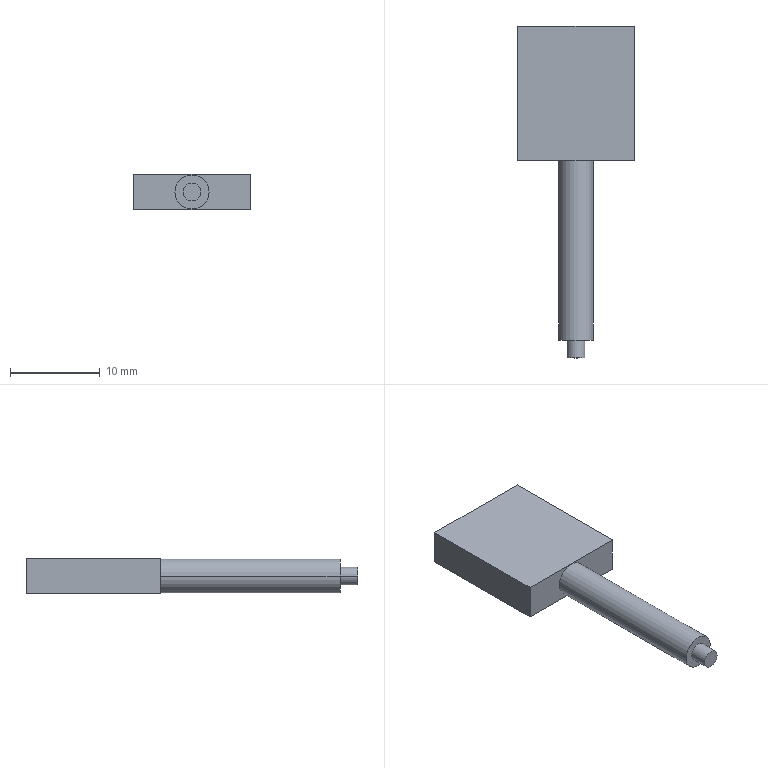Part | STEP file | 0246_008_FPCN14H-1 | 1 solid | 17 faces | box 13 x 37 x 4 mm | volume 994.356 mm3 | plane 13 | cylinder 4 | commonest cylinder face diameters 2 x2 3.8 x2
STEP:
#1=CARTESIAN_POINT('',(0.,0.,0.));
#2=DIRECTION('',(0.,0.,1.));
#3=DIRECTION('',(1.,0.,0.));
#4=AXIS2_PLACEMENT_3D('',#1,#2,#3);
#5=CARTESIAN_POINT('',(1.,-37.,0.));
#6=VERTEX_POINT('',#5);
#7=CARTESIAN_POINT('',(-1.,-37.,0.));
#8=VERTEX_POINT('',#7);
#9=CARTESIAN_POINT('',(0.,-37.,0.));
#10=DIRECTION('',(0.,-1.,0.));
#11=DIRECTION('',(1.,0.,0.));
#12=AXIS2_PLACEMENT_3D('',#9,#10,#11);
#13=CIRCLE('',#12,1.);
#14=CARTESIAN_POINT('',(0.,-37.,0.));
#15=DIRECTION('',(0.,1.,0.));
#16=DIRECTION('',(-1.,0.,0.));
#17=AXIS2_PLACEMENT_3D('',#14,#15,#16);
#18=CYLINDRICAL_SURFACE('',#17,1.);
#19=CARTESIAN_POINT('',(3.142,0.));
#20=DIRECTION('',(-1.,0.));
#21=VECTOR('',#20,1.);
#22=LINE('',#19,#21);
#23=(GEOMETRIC_REPRESENTATION_CONTEXT(2)PARAMETRIC_REPRESENTATION_CONTEXT()REPRESENTATION_CONTEXT('',''));
#24=DEFINITIONAL_REPRESENTATION('',(#22),#23);
#25=PCURVE('',#18,#24);
#26=CARTESIAN_POINT('',(0.,-37.,0.));
#27=DIRECTION('',(0.,-1.,0.));
#28=DIRECTION('',(1.,0.,0.));
#29=AXIS2_PLACEMENT_3D('',#26,#27,#28);
#30=PLANE('',#29);
#31=CARTESIAN_POINT('',(0.,0.));
#32=DIRECTION('',(1.,0.));
#33=AXIS2_PLACEMENT_2D('',#31,#32);
#34=CIRCLE('',#33,1.);
#35=(GEOMETRIC_REPRESENTATION_CONTEXT(2)PARAMETRIC_REPRESENTATION_CONTEXT()REPRESENTATION_CONTEXT('',''));
#36=DEFINITIONAL_REPRESENTATION('',(#34),#35);
#37=PCURVE('',#30,#36);
#38=SURFACE_CURVE('',#13,(#25,#37),.PCURVE_S1.);
#39=EDGE_CURVE('',#6,#8,#38,.T.);
#40=ORIENTED_EDGE('',*,*,#39,.F.);
#41=CARTESIAN_POINT('',(1.,-35.,0.));
#42=VERTEX_POINT('',#41);
#43=CARTESIAN_POINT('',(1.,-37.,0.));
#44=DIRECTION('',(0.,1.,0.));
#45=VECTOR('',#44,1.);
#46=LINE('',#43,#45);
#47=CARTESIAN_POINT('',(3.142,0.));
#48=DIRECTION('',(0.,1.));
#49=VECTOR('',#48,1.);
#50=LINE('',#47,#49);
#51=(GEOMETRIC_REPRESENTATION_CONTEXT(2)PARAMETRIC_REPRESENTATION_CONTEXT()REPRESENTATION_CONTEXT('',''));
#52=DEFINITIONAL_REPRESENTATION('',(#50),#51);
#53=PCURVE('',#18,#52);
#54=CARTESIAN_POINT('',(0.,-37.,0.));
#55=DIRECTION('',(0.,1.,0.));
#56=DIRECTION('',(-1.,0.,0.));
#57=AXIS2_PLACEMENT_3D('',#54,#55,#56);
#58=CYLINDRICAL_SURFACE('',#57,1.);
#59=CARTESIAN_POINT('',(3.142,0.));
#60=DIRECTION('',(0.,1.));
#61=VECTOR('',#60,1.);
#62=LINE('',#59,#61);
#63=(GEOMETRIC_REPRESENTATION_CONTEXT(2)PARAMETRIC_REPRESENTATION_CONTEXT()REPRESENTATION_CONTEXT('',''));
#64=DEFINITIONAL_REPRESENTATION('',(#62),#63);
#65=PCURVE('',#58,#64);
#66=SURFACE_CURVE('',#46,(#53,#65),.PCURVE_S1.);
#67=EDGE_CURVE('',#6,#42,#66,.T.);
#68=ORIENTED_EDGE('',*,*,#67,.T.);
#69=CARTESIAN_POINT('',(-1.,-35.,0.));
#70=VERTEX_POINT('',#69);
#71=CARTESIAN_POINT('',(0.,-35.,0.));
#72=DIRECTION('',(0.,-1.,0.));
#73=DIRECTION('',(1.,0.,0.));
#74=AXIS2_PLACEMENT_3D('',#71,#72,#73);
#75=CIRCLE('',#74,1.);
#76=CARTESIAN_POINT('',(3.142,2.));
#77=DIRECTION('',(-1.,0.));
#78=VECTOR('',#77,1.);
#79=LINE('',#76,#78);
#80=(GEOMETRIC_REPRESENTATION_CONTEXT(2)PARAMETRIC_REPRESENTATION_CONTEXT()REPRESENTATION_CONTEXT('',''));
#81=DEFINITIONAL_REPRESENTATION('',(#79),#80);
#82=PCURVE('',#18,#81);
#83=CARTESIAN_POINT('',(0.,-35.,0.));
#84=DIRECTION('',(0.,-1.,0.));
#85=DIRECTION('',(1.,0.,0.));
#86=AXIS2_PLACEMENT_3D('',#83,#84,#85);
#87=PLANE('',#86);
#88=CARTESIAN_POINT('',(0.,0.));
#89=DIRECTION('',(1.,0.));
#90=AXIS2_PLACEMENT_2D('',#88,#89);
#91=CIRCLE('',#90,1.);
#92=(GEOMETRIC_REPRESENTATION_CONTEXT(2)PARAMETRIC_REPRESENTATION_CONTEXT()REPRESENTATION_CONTEXT('',''));
#93=DEFINITIONAL_REPRESENTATION('',(#91),#92);
#94=PCURVE('',#87,#93);
#95=SURFACE_CURVE('',#75,(#82,#94),.PCURVE_S1.);
#96=EDGE_CURVE('',#42,#70,#95,.T.);
#97=ORIENTED_EDGE('',*,*,#96,.T.);
#98=CARTESIAN_POINT('',(-1.,-37.,0.));
#99=DIRECTION('',(0.,1.,0.));
#100=VECTOR('',#99,1.);
#101=LINE('',#98,#100);
#102=CARTESIAN_POINT('',(0.,0.));
#103=DIRECTION('',(0.,1.));
#104=VECTOR('',#103,1.);
#105=LINE('',#102,#104);
#106=(GEOMETRIC_REPRESENTATION_CONTEXT(2)PARAMETRIC_REPRESENTATION_CONTEXT()REPRESENTATION_CONTEXT('',''));
#107=DEFINITIONAL_REPRESENTATION('',(#105),#106);
#108=PCURVE('',#18,#107);
#109=CARTESIAN_POINT('',(6.283,0.));
#110=DIRECTION('',(0.,1.));
#111=VECTOR('',#110,1.);
#112=LINE('',#109,#111);
#113=(GEOMETRIC_REPRESENTATION_CONTEXT(2)PARAMETRIC_REPRESENTATION_CONTEXT()REPRESENTATION_CONTEXT('',''));
#114=DEFINITIONAL_REPRESENTATION('',(#112),#113);
#115=PCURVE('',#58,#114);
#116=SURFACE_CURVE('',#101,(#108,#115),.PCURVE_S1.);
#117=EDGE_CURVE('',#8,#70,#116,.T.);
#118=ORIENTED_EDGE('',*,*,#117,.F.);
#119=EDGE_LOOP('',(#40,#68,#97,#118));
#120=FACE_BOUND('',#119,.T.);
#121=ADVANCED_FACE('',(#120),#18,.T.);
#122=CARTESIAN_POINT('',(1.9,-35.,0.));
#123=VERTEX_POINT('',#122);
#124=CARTESIAN_POINT('',(-1.9,-35.,0.));
#125=VERTEX_POINT('',#124);
#126=CARTESIAN_POINT('',(0.,-35.,0.));
#127=DIRECTION('',(0.,-1.,0.));
#128=DIRECTION('',(1.,0.,0.));
#129=AXIS2_PLACEMENT_3D('',#126,#127,#128);
#130=CIRCLE('',#129,1.9);
#131=CARTESIAN_POINT('',(0.,-35.,0.));
#132=DIRECTION('',(0.,1.,0.));
#133=DIRECTION('',(-1.,0.,0.));
#134=AXIS2_PLACEMENT_3D('',#131,#132,#133);
#135=CYLINDRICAL_SURFACE('',#134,1.9);
#136=CARTESIAN_POINT('',(3.142,0.));
#137=DIRECTION('',(-1.,0.));
#138=VECTOR('',#137,1.);
#139=LINE('',#136,#138);
#140=(GEOMETRIC_REPRESENTATION_CONTEXT(2)PARAMETRIC_REPRESENTATION_CONTEXT()REPRESENTATION_CONTEXT('',''));
#141=DEFINITIONAL_REPRESENTATION('',(#139),#140);
#142=PCURVE('',#135,#141);
#143=CARTESIAN_POINT('',(0.,0.));
#144=DIRECTION('',(1.,0.));
#145=AXIS2_PLACEMENT_2D('',#143,#144);
#146=CIRCLE('',#145,1.9);
#147=(GEOMETRIC_REPRESENTATION_CONTEXT(2)PARAMETRIC_REPRESENTATION_CONTEXT()REPRESENTATION_CONTEXT('',''));
#148=DEFINITIONAL_REPRESENTATION('',(#146),#147);
#149=PCURVE('',#87,#148);
#150=SURFACE_CURVE('',#130,(#142,#149),.PCURVE_S1.);
#151=EDGE_CURVE('',#123,#125,#150,.T.);
#152=ORIENTED_EDGE('',*,*,#151,.F.);
#153=CARTESIAN_POINT('',(1.9,-15.,0.));
#154=VERTEX_POINT('',#153);
#155=CARTESIAN_POINT('',(1.9,-35.,0.));
#156=DIRECTION('',(0.,1.,0.));
#157=VECTOR('',#156,1.);
#158=LINE('',#155,#157);
#159=CARTESIAN_POINT('',(3.142,0.));
#160=DIRECTION('',(0.,1.));
#161=VECTOR('',#160,1.);
#162=LINE('',#159,#161);
#163=(GEOMETRIC_REPRESENTATION_CONTEXT(2)PARAMETRIC_REPRESENTATION_CONTEXT()REPRESENTATION_CONTEXT('',''));
#164=DEFINITIONAL_REPRESENTATION('',(#162),#163);
#165=PCURVE('',#135,#164);
#166=CARTESIAN_POINT('',(0.,-35.,0.));
#167=DIRECTION('',(0.,1.,0.));
#168=DIRECTION('',(-1.,0.,0.));
#169=AXIS2_PLACEMENT_3D('',#166,#167,#168);
#170=CYLINDRICAL_SURFACE('',#169,1.9);
#171=CARTESIAN_POINT('',(3.142,0.));
#172=DIRECTION('',(0.,1.));
#173=VECTOR('',#172,1.);
#174=LINE('',#171,#173);
#175=(GEOMETRIC_REPRESENTATION_CONTEXT(2)PARAMETRIC_REPRESENTATION_CONTEXT()REPRESENTATION_CONTEXT('',''));
#176=DEFINITIONAL_REPRESENTATION('',(#174),#175);
#177=PCURVE('',#170,#176);
#178=SURFACE_CURVE('',#158,(#165,#177),.PCURVE_S1.);
#179=EDGE_CURVE('',#123,#154,#178,.T.);
#180=ORIENTED_EDGE('',*,*,#179,.T.);
#181=CARTESIAN_POINT('',(-1.9,-15.,0.));
#182=VERTEX_POINT('',#181);
#183=CARTESIAN_POINT('',(0.,-15.,0.));
#184=DIRECTION('',(0.,-1.,0.));
#185=DIRECTION('',(-1.,0.,0.));
#186=AXIS2_PLACEMENT_3D('',#183,#184,#185);
#187=CIRCLE('',#186,1.9);
#188=CARTESIAN_POINT('',(6.283,20.));
#189=DIRECTION('',(-1.,0.));
#190=VECTOR('',#189,1.);
#191=LINE('',#188,#190);
#192=(GEOMETRIC_REPRESENTATION_CONTEXT(2)PARAMETRIC_REPRESENTATION_CONTEXT()REPRESENTATION_CONTEXT('',''));
#193=DEFINITIONAL_REPRESENTATION('',(#191),#192);
#194=PCURVE('',#135,#193);
#195=CARTESIAN_POINT('',(-6.5,-15.,2.));
#196=DIRECTION('',(0.,1.,0.));
#197=DIRECTION('',(-1.,0.,0.));
#198=AXIS2_PLACEMENT_3D('',#195,#196,#197);
#199=PLANE('',#198);
#200=CARTESIAN_POINT('',(-4.6,-2.));
#201=CARTESIAN_POINT('',(-4.6,-5.291));
#202=CARTESIAN_POINT('',(-7.45,-3.645));
#203=CARTESIAN_POINT('',(-10.3,-2.));
#204=CARTESIAN_POINT('',(-7.45,-0.3546));
#205=CARTESIAN_POINT('',(-4.6,1.291));
#206=CARTESIAN_POINT('',(-4.6,-2.));
#207=(BOUNDED_CURVE()B_SPLINE_CURVE(2,(#200,#201,#202,#203,#204,#205,#206),.UNSPECIFIED.,.T.,.F.)B_SPLINE_CURVE_WITH_KNOTS((1,2,2,2,2,1),(-2.094,0.,2.094,4.189,6.283,8.378),.UNSPECIFIED.)CURVE()GEOMETRIC_REPRESENTATION_ITEM()RATIONAL_B_SPLINE_CURVE((1.,0.5,1.,0.5,1.,0.5,1.))REPRESENTATION_ITEM(''));
#208=(GEOMETRIC_REPRESENTATION_CONTEXT(2)PARAMETRIC_REPRESENTATION_CONTEXT()REPRESENTATION_CONTEXT('',''));
#209=DEFINITIONAL_REPRESENTATION('',(#207),#208);
#210=PCURVE('',#199,#209);
#211=SURFACE_CURVE('',#187,(#194,#210),.PCURVE_S1.);
#212=EDGE_CURVE('',#154,#182,#211,.T.);
#213=ORIENTED_EDGE('',*,*,#212,.T.);
#214=CARTESIAN_POINT('',(-1.9,-35.,0.));
#215=DIRECTION('',(0.,1.,0.));
#216=VECTOR('',#215,1.);
#217=LINE('',#214,#216);
#218=CARTESIAN_POINT('',(0.,0.));
#219=DIRECTION('',(0.,1.));
#220=VECTOR('',#219,1.);
#221=LINE('',#218,#220);
#222=(GEOMETRIC_REPRESENTATION_CONTEXT(2)PARAMETRIC_REPRESENTATION_CONTEXT()REPRESENTATION_CONTEXT('',''));
#223=DEFINITIONAL_REPRESENTATION('',(#221),#222);
#224=PCURVE('',#135,#223);
#225=CARTESIAN_POINT('',(6.283,0.));
#226=DIRECTION('',(0.,1.));
#227=VECTOR('',#226,1.);
#228=LINE('',#225,#227);
#229=(GEOMETRIC_REPRESENTATION_CONTEXT(2)PARAMETRIC_REPRESENTATION_CONTEXT()REPRESENTATION_CONTEXT('',''));
#230=DEFINITIONAL_REPRESENTATION('',(#228),#229);
#231=PCURVE('',#170,#230);
#232=SURFACE_CURVE('',#217,(#224,#231),.PCURVE_S1.);
#233=EDGE_CURVE('',#125,#182,#232,.T.);
#234=ORIENTED_EDGE('',*,*,#233,.F.);
#235=EDGE_LOOP('',(#152,#180,#213,#234));
#236=FACE_BOUND('',#235,.T.);
#237=ADVANCED_FACE('',(#236),#135,.T.);
#238=CARTESIAN_POINT('',(0.,-35.,0.));
#239=DIRECTION('',(0.,-1.,0.));
#240=DIRECTION('',(1.,0.,0.));
#241=AXIS2_PLACEMENT_3D('',#238,#239,#240);
#242=CIRCLE('',#241,1.9);
#243=CARTESIAN_POINT('',(0.,0.));
#244=DIRECTION('',(1.,0.));
#245=AXIS2_PLACEMENT_2D('',#243,#244);
#246=CIRCLE('',#245,1.9);
#247=(GEOMETRIC_REPRESENTATION_CONTEXT(2)PARAMETRIC_REPRESENTATION_CONTEXT()REPRESENTATION_CONTEXT('',''));
#248=DEFINITIONAL_REPRESENTATION('',(#246),#247);
#249=PCURVE('',#87,#248);
#250=CARTESIAN_POINT('',(9.425,0.));
#251=DIRECTION('',(-1.,0.));
#252=VECTOR('',#251,1.);
#253=LINE('',#250,#252);
#254=(GEOMETRIC_REPRESENTATION_CONTEXT(2)PARAMETRIC_REPRESENTATION_CONTEXT()REPRESENTATION_CONTEXT('',''));
#255=DEFINITIONAL_REPRESENTATION('',(#253),#254);
#256=PCURVE('',#170,#255);
#257=SURFACE_CURVE('',#242,(#249,#256),.PCURVE_S1.);
#258=EDGE_CURVE('',#125,#123,#257,.T.);
#259=ORIENTED_EDGE('',*,*,#258,.T.);
#260=ORIENTED_EDGE('',*,*,#151,.T.);
#261=EDGE_LOOP('',(#259,#260));
#262=FACE_BOUND('',#261,.T.);
#263=CARTESIAN_POINT('',(0.,-35.,0.));
#264=DIRECTION('',(0.,-1.,0.));
#265=DIRECTION('',(1.,0.,0.));
#266=AXIS2_PLACEMENT_3D('',#263,#264,#265);
#267=CIRCLE('',#266,1.);
#268=CARTESIAN_POINT('',(0.,0.));
#269=DIRECTION('',(1.,0.));
#270=AXIS2_PLACEMENT_2D('',#268,#269);
#271=CIRCLE('',#270,1.);
#272=(GEOMETRIC_REPRESENTATION_CONTEXT(2)PARAMETRIC_REPRESENTATION_CONTEXT()REPRESENTATION_CONTEXT('',''));
#273=DEFINITIONAL_REPRESENTATION('',(#271),#272);
#274=PCURVE('',#87,#273);
#275=CARTESIAN_POINT('',(9.425,2.));
#276=DIRECTION('',(-1.,0.));
#277=VECTOR('',#276,1.);
#278=LINE('',#275,#277);
#279=(GEOMETRIC_REPRESENTATION_CONTEXT(2)PARAMETRIC_REPRESENTATION_CONTEXT()REPRESENTATION_CONTEXT('',''));
#280=DEFINITIONAL_REPRESENTATION('',(#278),#279);
#281=PCURVE('',#58,#280);
#282=SURFACE_CURVE('',#267,(#274,#281),.PCURVE_S1.);
#283=EDGE_CURVE('',#70,#42,#282,.T.);
#284=ORIENTED_EDGE('',*,*,#283,.F.);
#285=ORIENTED_EDGE('',*,*,#96,.F.);
#286=EDGE_LOOP('',(#284,#285));
#287=FACE_BOUND('',#286,.T.);
#288=ADVANCED_FACE('',(#262,#287),#87,.T.);
#289=CARTESIAN_POINT('',(-6.5,-15.,-2.));
#290=VERTEX_POINT('',#289);
#291=CARTESIAN_POINT('',(6.5,-15.,-2.));
#292=VERTEX_POINT('',#291);
#293=CARTESIAN_POINT('',(-6.5,-15.,-2.));
#294=DIRECTION('',(1.,0.,0.));
#295=VECTOR('',#294,1.);
#296=LINE('',#293,#295);
#297=CARTESIAN_POINT('',(0.,-4.));
#298=DIRECTION('',(-1.,0.));
#299=VECTOR('',#298,1.);
#300=LINE('',#297,#299);
#301=(GEOMETRIC_REPRESENTATION_CONTEXT(2)PARAMETRIC_REPRESENTATION_CONTEXT()REPRESENTATION_CONTEXT('',''));
#302=DEFINITIONAL_REPRESENTATION('',(#300),#301);
#303=PCURVE('',#199,#302);
#304=CARTESIAN_POINT('',(-6.5,-15.,-2.));
#305=DIRECTION('',(0.,0.,1.));
#306=DIRECTION('',(1.,0.,0.));
#307=AXIS2_PLACEMENT_3D('',#304,#305,#306);
#308=PLANE('',#307);
#309=CARTESIAN_POINT('',(0.,0.));
#310=DIRECTION('',(1.,0.));
#311=VECTOR('',#310,1.);
#312=LINE('',#309,#311);
#313=(GEOMETRIC_REPRESENTATION_CONTEXT(2)PARAMETRIC_REPRESENTATION_CONTEXT()REPRESENTATION_CONTEXT('',''));
#314=DEFINITIONAL_REPRESENTATION('',(#312),#313);
#315=PCURVE('',#308,#314);
#316=SURFACE_CURVE('',#296,(#303,#315),.PCURVE_S1.);
#317=EDGE_CURVE('',#290,#292,#316,.T.);
#318=ORIENTED_EDGE('',*,*,#317,.T.);
#319=CARTESIAN_POINT('',(6.5,-15.,2.));
#320=VERTEX_POINT('',#319);
#321=CARTESIAN_POINT('',(6.5,-15.,2.));
#322=DIRECTION('',(0.,0.,-1.));
#323=VECTOR('',#322,1.);
#324=LINE('',#321,#323);
#325=CARTESIAN_POINT('',(-13.,0.));
#326=DIRECTION('',(0.,-1.));
#327=VECTOR('',#326,1.);
#328=LINE('',#325,#327);
#329=(GEOMETRIC_REPRESENTATION_CONTEXT(2)PARAMETRIC_REPRESENTATION_CONTEXT()REPRESENTATION_CONTEXT('',''));
#330=DEFINITIONAL_REPRESENTATION('',(#328),#329);
#331=PCURVE('',#199,#330);
#332=CARTESIAN_POINT('',(6.5,0.,2.));
#333=DIRECTION('',(-1.,0.,0.));
#334=DIRECTION('',(0.,-1.,0.));
#335=AXIS2_PLACEMENT_3D('',#332,#333,#334);
#336=PLANE('',#335);
#337=CARTESIAN_POINT('',(15.,0.));
#338=DIRECTION('',(0.,-1.));
#339=VECTOR('',#338,1.);
#340=LINE('',#337,#339);
#341=(GEOMETRIC_REPRESENTATION_CONTEXT(2)PARAMETRIC_REPRESENTATION_CONTEXT()REPRESENTATION_CONTEXT('',''));
#342=DEFINITIONAL_REPRESENTATION('',(#340),#341);
#343=PCURVE('',#336,#342);
#344=SURFACE_CURVE('',#324,(#331,#343),.PCURVE_S1.);
#345=EDGE_CURVE('',#320,#292,#344,.T.);
#346=ORIENTED_EDGE('',*,*,#345,.F.);
#347=CARTESIAN_POINT('',(-6.5,-15.,2.));
#348=VERTEX_POINT('',#347);
#349=CARTESIAN_POINT('',(-6.5,-15.,2.));
#350=DIRECTION('',(1.,0.,0.));
#351=VECTOR('',#350,1.);
#352=LINE('',#349,#351);
#353=CARTESIAN_POINT('',(0.,0.));
#354=DIRECTION('',(-1.,0.));
#355=VECTOR('',#354,1.);
#356=LINE('',#353,#355);
#357=(GEOMETRIC_REPRESENTATION_CONTEXT(2)PARAMETRIC_REPRESENTATION_CONTEXT()REPRESENTATION_CONTEXT('',''));
#358=DEFINITIONAL_REPRESENTATION('',(#356),#357);
#359=PCURVE('',#199,#358);
#360=CARTESIAN_POINT('',(-6.5,-15.,2.));
#361=DIRECTION('',(0.,0.,1.));
#362=DIRECTION('',(1.,0.,0.));
#363=AXIS2_PLACEMENT_3D('',#360,#361,#362);
#364=PLANE('',#363);
#365=CARTESIAN_POINT('',(0.,0.));
#366=DIRECTION('',(1.,0.));
#367=VECTOR('',#366,1.);
#368=LINE('',#365,#367);
#369=(GEOMETRIC_REPRESENTATION_CONTEXT(2)PARAMETRIC_REPRESENTATION_CONTEXT()REPRESENTATION_CONTEXT('',''));
#370=DEFINITIONAL_REPRESENTATION('',(#368),#369);
#371=PCURVE('',#364,#370);
#372=SURFACE_CURVE('',#352,(#359,#371),.PCURVE_S1.);
#373=EDGE_CURVE('',#348,#320,#372,.T.);
#374=ORIENTED_EDGE('',*,*,#373,.F.);
#375=CARTESIAN_POINT('',(-6.5,-15.,2.));
#376=DIRECTION('',(0.,0.,-1.));
#377=VECTOR('',#376,1.);
#378=LINE('',#375,#377);
#379=CARTESIAN_POINT('',(0.,0.));
#380=DIRECTION('',(0.,-1.));
#381=VECTOR('',#380,1.);
#382=LINE('',#379,#381);
#383=(GEOMETRIC_REPRESENTATION_CONTEXT(2)PARAMETRIC_REPRESENTATION_CONTEXT()REPRESENTATION_CONTEXT('',''));
#384=DEFINITIONAL_REPRESENTATION('',(#382),#383);
#385=PCURVE('',#199,#384);
#386=CARTESIAN_POINT('',(-6.5,0.,2.));
#387=DIRECTION('',(1.,0.,0.));
#388=DIRECTION('',(0.,1.,0.));
#389=AXIS2_PLACEMENT_3D('',#386,#387,#388);
#390=PLANE('',#389);
#391=CARTESIAN_POINT('',(-15.,0.));
#392=DIRECTION('',(0.,-1.));
#393=VECTOR('',#392,1.);
#394=LINE('',#391,#393);
#395=(GEOMETRIC_REPRESENTATION_CONTEXT(2)PARAMETRIC_REPRESENTATION_CONTEXT()REPRESENTATION_CONTEXT('',''));
#396=DEFINITIONAL_REPRESENTATION('',(#394),#395);
#397=PCURVE('',#390,#396);
#398=SURFACE_CURVE('',#378,(#385,#397),.PCURVE_S1.);
#399=EDGE_CURVE('',#348,#290,#398,.T.);
#400=ORIENTED_EDGE('',*,*,#399,.T.);
#401=EDGE_LOOP('',(#318,#346,#374,#400));
#402=FACE_BOUND('',#401,.T.);
#403=CARTESIAN_POINT('',(0.,-15.,0.));
#404=DIRECTION('',(0.,-1.,0.));
#405=DIRECTION('',(-1.,0.,0.));
#406=AXIS2_PLACEMENT_3D('',#403,#404,#405);
#407=CIRCLE('',#406,1.9);
#408=CARTESIAN_POINT('',(-4.6,-2.));
#409=CARTESIAN_POINT('',(-4.6,-5.291));
#410=CARTESIAN_POINT('',(-7.45,-3.645));
#411=CARTESIAN_POINT('',(-10.3,-2.));
#412=CARTESIAN_POINT('',(-7.45,-0.3546));
#413=CARTESIAN_POINT('',(-4.6,1.291));
#414=CARTESIAN_POINT('',(-4.6,-2.));
#415=(BOUNDED_CURVE()B_SPLINE_CURVE(2,(#408,#409,#410,#411,#412,#413,#414),.UNSPECIFIED.,.T.,.F.)B_SPLINE_CURVE_WITH_KNOTS((1,2,2,2,2,1),(-2.094,0.,2.094,4.189,6.283,8.378),.UNSPECIFIED.)CURVE()GEOMETRIC_REPRESENTATION_ITEM()RATIONAL_B_SPLINE_CURVE((1.,0.5,1.,0.5,1.,0.5,1.))REPRESENTATION_ITEM(''));
#416=(GEOMETRIC_REPRESENTATION_CONTEXT(2)PARAMETRIC_REPRESENTATION_CONTEXT()REPRESENTATION_CONTEXT('',''));
#417=DEFINITIONAL_REPRESENTATION('',(#415),#416);
#418=PCURVE('',#199,#417);
#419=CARTESIAN_POINT('',(6.283,20.));
#420=DIRECTION('',(-1.,0.));
#421=VECTOR('',#420,1.);
#422=LINE('',#419,#421);
#423=(GEOMETRIC_REPRESENTATION_CONTEXT(2)PARAMETRIC_REPRESENTATION_CONTEXT()REPRESENTATION_CONTEXT('',''));
#424=DEFINITIONAL_REPRESENTATION('',(#422),#423);
#425=PCURVE('',#170,#424);
#426=SURFACE_CURVE('',#407,(#418,#425),.PCURVE_S1.);
#427=EDGE_CURVE('',#182,#154,#426,.T.);
#428=ORIENTED_EDGE('',*,*,#427,.F.);
#429=ORIENTED_EDGE('',*,*,#212,.F.);
#430=EDGE_LOOP('',(#428,#429));
#431=FACE_BOUND('',#430,.T.);
#432=ADVANCED_FACE('',(#402,#431),#199,.F.);
#433=CARTESIAN_POINT('',(-6.5,0.,-2.));
#434=VERTEX_POINT('',#433);
#435=CARTESIAN_POINT('',(-6.5,0.,-2.));
#436=DIRECTION('',(0.,-1.,0.));
#437=VECTOR('',#436,1.);
#438=LINE('',#435,#437);
#439=CARTESIAN_POINT('',(0.,-4.));
#440=DIRECTION('',(-1.,0.));
#441=VECTOR('',#440,1.);
#442=LINE('',#439,#441);
#443=(GEOMETRIC_REPRESENTATION_CONTEXT(2)PARAMETRIC_REPRESENTATION_CONTEXT()REPRESENTATION_CONTEXT('',''));
#444=DEFINITIONAL_REPRESENTATION('',(#442),#443);
#445=PCURVE('',#390,#444);
#446=CARTESIAN_POINT('',(0.,15.));
#447=DIRECTION('',(0.,-1.));
#448=VECTOR('',#447,1.);
#449=LINE('',#446,#448);
#450=(GEOMETRIC_REPRESENTATION_CONTEXT(2)PARAMETRIC_REPRESENTATION_CONTEXT()REPRESENTATION_CONTEXT('',''));
#451=DEFINITIONAL_REPRESENTATION('',(#449),#450);
#452=PCURVE('',#308,#451);
#453=SURFACE_CURVE('',#438,(#445,#452),.PCURVE_S1.);
#454=EDGE_CURVE('',#434,#290,#453,.T.);
#455=ORIENTED_EDGE('',*,*,#454,.T.);
#456=ORIENTED_EDGE('',*,*,#399,.F.);
#457=CARTESIAN_POINT('',(-6.5,0.,2.));
#458=VERTEX_POINT('',#457);
#459=CARTESIAN_POINT('',(-6.5,0.,2.));
#460=DIRECTION('',(0.,-1.,0.));
#461=VECTOR('',#460,1.);
#462=LINE('',#459,#461);
#463=CARTESIAN_POINT('',(0.,0.));
#464=DIRECTION('',(-1.,0.));
#465=VECTOR('',#464,1.);
#466=LINE('',#463,#465);
#467=(GEOMETRIC_REPRESENTATION_CONTEXT(2)PARAMETRIC_REPRESENTATION_CONTEXT()REPRESENTATION_CONTEXT('',''));
#468=DEFINITIONAL_REPRESENTATION('',(#466),#467);
#469=PCURVE('',#390,#468);
#470=CARTESIAN_POINT('',(0.,15.));
#471=DIRECTION('',(0.,-1.));
#472=VECTOR('',#471,1.);
#473=LINE('',#470,#472);
#474=(GEOMETRIC_REPRESENTATION_CONTEXT(2)PARAMETRIC_REPRESENTATION_CONTEXT()REPRESENTATION_CONTEXT('',''));
#475=DEFINITIONAL_REPRESENTATION('',(#473),#474);
#476=PCURVE('',#364,#475);
#477=SURFACE_CURVE('',#462,(#469,#476),.PCURVE_S1.);
#478=EDGE_CURVE('',#458,#348,#477,.T.);
#479=ORIENTED_EDGE('',*,*,#478,.F.);
#480=CARTESIAN_POINT('',(-6.5,0.,2.));
#481=DIRECTION('',(0.,0.,-1.));
#482=VECTOR('',#481,1.);
#483=LINE('',#480,#482);
#484=CARTESIAN_POINT('',(0.,0.));
#485=DIRECTION('',(0.,-1.));
#486=VECTOR('',#485,1.);
#487=LINE('',#484,#486);
#488=(GEOMETRIC_REPRESENTATION_CONTEXT(2)PARAMETRIC_REPRESENTATION_CONTEXT()REPRESENTATION_CONTEXT('',''));
#489=DEFINITIONAL_REPRESENTATION('',(#487),#488);
#490=PCURVE('',#390,#489);
#491=CARTESIAN_POINT('',(-6.5,0.,2.));
#492=DIRECTION('',(0.,-1.,0.));
#493=DIRECTION('',(1.,0.,0.));
#494=AXIS2_PLACEMENT_3D('',#491,#492,#493);
#495=PLANE('',#494);
#496=CARTESIAN_POINT('',(0.,0.));
#497=DIRECTION('',(0.,-1.));
#498=VECTOR('',#497,1.);
#499=LINE('',#496,#498);
#500=(GEOMETRIC_REPRESENTATION_CONTEXT(2)PARAMETRIC_REPRESENTATION_CONTEXT()REPRESENTATION_CONTEXT('',''));
#501=DEFINITIONAL_REPRESENTATION('',(#499),#500);
#502=PCURVE('',#495,#501);
#503=SURFACE_CURVE('',#483,(#490,#502),.PCURVE_S1.);
#504=EDGE_CURVE('',#458,#434,#503,.T.);
#505=ORIENTED_EDGE('',*,*,#504,.T.);
#506=EDGE_LOOP('',(#455,#456,#479,#505));
#507=FACE_BOUND('',#506,.T.);
#508=ADVANCED_FACE('',(#507),#390,.F.);
#509=CARTESIAN_POINT('',(6.5,0.,-2.));
#510=VERTEX_POINT('',#509);
#511=CARTESIAN_POINT('',(6.5,0.,-2.));
#512=DIRECTION('',(0.,1.,0.));
#513=VECTOR('',#512,1.);
#514=LINE('',#511,#513);
#515=CARTESIAN_POINT('',(0.,-4.));
#516=DIRECTION('',(-1.,0.));
#517=VECTOR('',#516,1.);
#518=LINE('',#515,#517);
#519=(GEOMETRIC_REPRESENTATION_CONTEXT(2)PARAMETRIC_REPRESENTATION_CONTEXT()REPRESENTATION_CONTEXT('',''));
#520=DEFINITIONAL_REPRESENTATION('',(#518),#519);
#521=PCURVE('',#336,#520);
#522=CARTESIAN_POINT('',(13.,15.));
#523=DIRECTION('',(0.,1.));
#524=VECTOR('',#523,1.);
#525=LINE('',#522,#524);
#526=(GEOMETRIC_REPRESENTATION_CONTEXT(2)PARAMETRIC_REPRESENTATION_CONTEXT()REPRESENTATION_CONTEXT('',''));
#527=DEFINITIONAL_REPRESENTATION('',(#525),#526);
#528=PCURVE('',#308,#527);
#529=SURFACE_CURVE('',#514,(#521,#528),.PCURVE_S1.);
#530=EDGE_CURVE('',#292,#510,#529,.T.);
#531=ORIENTED_EDGE('',*,*,#530,.T.);
#532=CARTESIAN_POINT('',(6.5,0.,2.));
#533=VERTEX_POINT('',#532);
#534=CARTESIAN_POINT('',(6.5,0.,2.));
#535=DIRECTION('',(0.,0.,-1.));
#536=VECTOR('',#535,1.);
#537=LINE('',#534,#536);
#538=CARTESIAN_POINT('',(0.,0.));
#539=DIRECTION('',(0.,-1.));
#540=VECTOR('',#539,1.);
#541=LINE('',#538,#540);
#542=(GEOMETRIC_REPRESENTATION_CONTEXT(2)PARAMETRIC_REPRESENTATION_CONTEXT()REPRESENTATION_CONTEXT('',''));
#543=DEFINITIONAL_REPRESENTATION('',(#541),#542);
#544=PCURVE('',#336,#543);
#545=CARTESIAN_POINT('',(13.,0.));
#546=DIRECTION('',(0.,-1.));
#547=VECTOR('',#546,1.);
#548=LINE('',#545,#547);
#549=(GEOMETRIC_REPRESENTATION_CONTEXT(2)PARAMETRIC_REPRESENTATION_CONTEXT()REPRESENTATION_CONTEXT('',''));
#550=DEFINITIONAL_REPRESENTATION('',(#548),#549);
#551=PCURVE('',#495,#550);
#552=SURFACE_CURVE('',#537,(#544,#551),.PCURVE_S1.);
#553=EDGE_CURVE('',#533,#510,#552,.T.);
#554=ORIENTED_EDGE('',*,*,#553,.F.);
#555=CARTESIAN_POINT('',(6.5,0.,2.));
#556=DIRECTION('',(0.,1.,0.));
#557=VECTOR('',#556,1.);
#558=LINE('',#555,#557);
#559=CARTESIAN_POINT('',(0.,0.));
#560=DIRECTION('',(-1.,0.));
#561=VECTOR('',#560,1.);
#562=LINE('',#559,#561);
#563=(GEOMETRIC_REPRESENTATION_CONTEXT(2)PARAMETRIC_REPRESENTATION_CONTEXT()REPRESENTATION_CONTEXT('',''));
#564=DEFINITIONAL_REPRESENTATION('',(#562),#563);
#565=PCURVE('',#336,#564);
#566=CARTESIAN_POINT('',(13.,15.));
#567=DIRECTION('',(0.,1.));
#568=VECTOR('',#567,1.);
#569=LINE('',#566,#568);
#570=(GEOMETRIC_REPRESENTATION_CONTEXT(2)PARAMETRIC_REPRESENTATION_CONTEXT()REPRESENTATION_CONTEXT('',''));
#571=DEFINITIONAL_REPRESENTATION('',(#569),#570);
#572=PCURVE('',#364,#571);
#573=SURFACE_CURVE('',#558,(#565,#572),.PCURVE_S1.);
#574=EDGE_CURVE('',#320,#533,#573,.T.);
#575=ORIENTED_EDGE('',*,*,#574,.F.);
#576=ORIENTED_EDGE('',*,*,#345,.T.);
#577=EDGE_LOOP('',(#531,#554,#575,#576));
#578=FACE_BOUND('',#577,.T.);
#579=ADVANCED_FACE('',(#578),#336,.F.);
#580=CARTESIAN_POINT('',(6.25,0.,-0.15));
#581=VERTEX_POINT('',#580);
#582=CARTESIAN_POINT('',(-6.25,0.,-0.15));
#583=VERTEX_POINT('',#582);
#584=CARTESIAN_POINT('',(-6.25,0.,-0.15));
#585=DIRECTION('',(-1.,0.,0.));
#586=VECTOR('',#585,1.);
#587=LINE('',#584,#586);
#588=CARTESIAN_POINT('',(0.25,-2.15));
#589=DIRECTION('',(-1.,0.));
#590=VECTOR('',#589,1.);
#591=LINE('',#588,#590);
#592=(GEOMETRIC_REPRESENTATION_CONTEXT(2)PARAMETRIC_REPRESENTATION_CONTEXT()REPRESENTATION_CONTEXT('',''));
#593=DEFINITIONAL_REPRESENTATION('',(#591),#592);
#594=PCURVE('',#495,#593);
#595=CARTESIAN_POINT('',(-6.25,-5.,-0.15));
#596=DIRECTION('',(0.,0.,-1.));
#597=DIRECTION('',(-1.,0.,0.));
#598=AXIS2_PLACEMENT_3D('',#595,#596,#597);
#599=PLANE('',#598);
#600=CARTESIAN_POINT('',(0.,5.));
#601=DIRECTION('',(1.,0.));
#602=VECTOR('',#601,1.);
#603=LINE('',#600,#602);
#604=(GEOMETRIC_REPRESENTATION_CONTEXT(2)PARAMETRIC_REPRESENTATION_CONTEXT()REPRESENTATION_CONTEXT('',''));
#605=DEFINITIONAL_REPRESENTATION('',(#603),#604);
#606=PCURVE('',#599,#605);
#607=SURFACE_CURVE('',#587,(#594,#606),.PCURVE_S1.);
#608=EDGE_CURVE('',#581,#583,#607,.T.);
#609=ORIENTED_EDGE('',*,*,#608,.F.);
#610=CARTESIAN_POINT('',(6.25,0.,0.15));
#611=VERTEX_POINT('',#610);
#612=CARTESIAN_POINT('',(6.25,0.,0.15));
#613=DIRECTION('',(0.,0.,-1.));
#614=VECTOR('',#613,1.);
#615=LINE('',#612,#614);
#616=CARTESIAN_POINT('',(12.75,-1.85));
#617=DIRECTION('',(0.,-1.));
#618=VECTOR('',#617,1.);
#619=LINE('',#616,#618);
#620=(GEOMETRIC_REPRESENTATION_CONTEXT(2)PARAMETRIC_REPRESENTATION_CONTEXT()REPRESENTATION_CONTEXT('',''));
#621=DEFINITIONAL_REPRESENTATION('',(#619),#620);
#622=PCURVE('',#495,#621);
#623=CARTESIAN_POINT('',(6.25,-5.,0.15));
#624=DIRECTION('',(1.,0.,0.));
#625=DIRECTION('',(0.,1.,0.));
#626=AXIS2_PLACEMENT_3D('',#623,#624,#625);
#627=PLANE('',#626);
#628=CARTESIAN_POINT('',(5.,0.));
#629=DIRECTION('',(0.,-1.));
#630=VECTOR('',#629,1.);
#631=LINE('',#628,#630);
#632=(GEOMETRIC_REPRESENTATION_CONTEXT(2)PARAMETRIC_REPRESENTATION_CONTEXT()REPRESENTATION_CONTEXT('',''));
#633=DEFINITIONAL_REPRESENTATION('',(#631),#632);
#634=PCURVE('',#627,#633);
#635=SURFACE_CURVE('',#615,(#622,#634),.PCURVE_S1.);
#636=EDGE_CURVE('',#611,#581,#635,.T.);
#637=ORIENTED_EDGE('',*,*,#636,.F.);
#638=CARTESIAN_POINT('',(-6.25,0.,0.15));
#639=VERTEX_POINT('',#638);
#640=CARTESIAN_POINT('',(-6.25,0.,0.15));
#641=DIRECTION('',(1.,0.,0.));
#642=VECTOR('',#641,1.);
#643=LINE('',#640,#642);
#644=CARTESIAN_POINT('',(0.25,-1.85));
#645=DIRECTION('',(1.,0.));
#646=VECTOR('',#645,1.);
#647=LINE('',#644,#646);
#648=(GEOMETRIC_REPRESENTATION_CONTEXT(2)PARAMETRIC_REPRESENTATION_CONTEXT()REPRESENTATION_CONTEXT('',''));
#649=DEFINITIONAL_REPRESENTATION('',(#647),#648);
#650=PCURVE('',#495,#649);
#651=CARTESIAN_POINT('',(-6.25,-5.,0.15));
#652=DIRECTION('',(0.,0.,1.));
#653=DIRECTION('',(1.,0.,0.));
#654=AXIS2_PLACEMENT_3D('',#651,#652,#653);
#655=PLANE('',#654);
#656=CARTESIAN_POINT('',(0.,5.));
#657=DIRECTION('',(1.,0.));
#658=VECTOR('',#657,1.);
#659=LINE('',#656,#658);
#660=(GEOMETRIC_REPRESENTATION_CONTEXT(2)PARAMETRIC_REPRESENTATION_CONTEXT()REPRESENTATION_CONTEXT('',''));
#661=DEFINITIONAL_REPRESENTATION('',(#659),#660);
#662=PCURVE('',#655,#661);
#663=SURFACE_CURVE('',#643,(#650,#662),.PCURVE_S1.);
#664=EDGE_CURVE('',#639,#611,#663,.T.);
#665=ORIENTED_EDGE('',*,*,#664,.F.);
#666=CARTESIAN_POINT('',(-6.25,0.,0.15));
#667=DIRECTION('',(0.,0.,1.));
#668=VECTOR('',#667,1.);
#669=LINE('',#666,#668);
#670=CARTESIAN_POINT('',(0.25,-1.85));
#671=DIRECTION('',(0.,1.));
#672=VECTOR('',#671,1.);
#673=LINE('',#670,#672);
#674=(GEOMETRIC_REPRESENTATION_CONTEXT(2)PARAMETRIC_REPRESENTATION_CONTEXT()REPRESENTATION_CONTEXT('',''));
#675=DEFINITIONAL_REPRESENTATION('',(#673),#674);
#676=PCURVE('',#495,#675);
#677=CARTESIAN_POINT('',(-6.25,-5.,0.15));
#678=DIRECTION('',(-1.,0.,0.));
#679=DIRECTION('',(0.,-1.,0.));
#680=AXIS2_PLACEMENT_3D('',#677,#678,#679);
#681=PLANE('',#680);
#682=CARTESIAN_POINT('',(-5.,0.));
#683=DIRECTION('',(0.,1.));
#684=VECTOR('',#683,1.);
#685=LINE('',#682,#684);
#686=(GEOMETRIC_REPRESENTATION_CONTEXT(2)PARAMETRIC_REPRESENTATION_CONTEXT()REPRESENTATION_CONTEXT('',''));
#687=DEFINITIONAL_REPRESENTATION('',(#685),#686);
#688=PCURVE('',#681,#687);
#689=SURFACE_CURVE('',#669,(#676,#688),.PCURVE_S1.);
#690=EDGE_CURVE('',#583,#639,#689,.T.);
#691=ORIENTED_EDGE('',*,*,#690,.F.);
#692=EDGE_LOOP('',(#609,#637,#665,#691));
#693=FACE_BOUND('',#692,.T.);
#694=CARTESIAN_POINT('',(-6.5,0.,-2.));
#695=DIRECTION('',(-1.,0.,0.));
#696=VECTOR('',#695,1.);
#697=LINE('',#694,#696);
#698=CARTESIAN_POINT('',(0.,-4.));
#699=DIRECTION('',(-1.,0.));
#700=VECTOR('',#699,1.);
#701=LINE('',#698,#700);
#702=(GEOMETRIC_REPRESENTATION_CONTEXT(2)PARAMETRIC_REPRESENTATION_CONTEXT()REPRESENTATION_CONTEXT('',''));
#703=DEFINITIONAL_REPRESENTATION('',(#701),#702);
#704=PCURVE('',#495,#703);
#705=CARTESIAN_POINT('',(0.,15.));
#706=DIRECTION('',(-1.,0.));
#707=VECTOR('',#706,1.);
#708=LINE('',#705,#707);
#709=(GEOMETRIC_REPRESENTATION_CONTEXT(2)PARAMETRIC_REPRESENTATION_CONTEXT()REPRESENTATION_CONTEXT('',''));
#710=DEFINITIONAL_REPRESENTATION('',(#708),#709);
#711=PCURVE('',#308,#710);
#712=SURFACE_CURVE('',#697,(#704,#711),.PCURVE_S1.);
#713=EDGE_CURVE('',#510,#434,#712,.T.);
#714=ORIENTED_EDGE('',*,*,#713,.T.);
#715=ORIENTED_EDGE('',*,*,#504,.F.);
#716=CARTESIAN_POINT('',(-6.5,0.,2.));
#717=DIRECTION('',(-1.,0.,0.));
#718=VECTOR('',#717,1.);
#719=LINE('',#716,#718);
#720=CARTESIAN_POINT('',(0.,0.));
#721=DIRECTION('',(-1.,0.));
#722=VECTOR('',#721,1.);
#723=LINE('',#720,#722);
#724=(GEOMETRIC_REPRESENTATION_CONTEXT(2)PARAMETRIC_REPRESENTATION_CONTEXT()REPRESENTATION_CONTEXT('',''));
#725=DEFINITIONAL_REPRESENTATION('',(#723),#724);
#726=PCURVE('',#495,#725);
#727=CARTESIAN_POINT('',(0.,15.));
#728=DIRECTION('',(-1.,0.));
#729=VECTOR('',#728,1.);
#730=LINE('',#727,#729);
#731=(GEOMETRIC_REPRESENTATION_CONTEXT(2)PARAMETRIC_REPRESENTATION_CONTEXT()REPRESENTATION_CONTEXT('',''));
#732=DEFINITIONAL_REPRESENTATION('',(#730),#731);
#733=PCURVE('',#364,#732);
#734=SURFACE_CURVE('',#719,(#726,#733),.PCURVE_S1.);
#735=EDGE_CURVE('',#533,#458,#734,.T.);
#736=ORIENTED_EDGE('',*,*,#735,.F.);
#737=ORIENTED_EDGE('',*,*,#553,.T.);
#738=EDGE_LOOP('',(#714,#715,#736,#737));
#739=FACE_BOUND('',#738,.T.);
#740=ADVANCED_FACE('',(#693,#739),#495,.F.);
#741=ORIENTED_EDGE('',*,*,#478,.T.);
#742=ORIENTED_EDGE('',*,*,#373,.T.);
#743=ORIENTED_EDGE('',*,*,#574,.T.);
#744=ORIENTED_EDGE('',*,*,#735,.T.);
#745=EDGE_LOOP('',(#741,#742,#743,#744));
#746=FACE_BOUND('',#745,.T.);
#747=ADVANCED_FACE('',(#746),#364,.T.);
#748=ORIENTED_EDGE('',*,*,#454,.F.);
#749=ORIENTED_EDGE('',*,*,#713,.F.);
#750=ORIENTED_EDGE('',*,*,#530,.F.);
#751=ORIENTED_EDGE('',*,*,#317,.F.);
#752=EDGE_LOOP('',(#748,#749,#750,#751));
#753=FACE_BOUND('',#752,.T.);
#754=ADVANCED_FACE('',(#753),#308,.F.);
#755=ORIENTED_EDGE('',*,*,#636,.T.);
#756=CARTESIAN_POINT('',(6.25,-5.,-0.15));
#757=VERTEX_POINT('',#756);
#758=CARTESIAN_POINT('',(6.25,-5.,-0.15));
#759=DIRECTION('',(0.,1.,0.));
#760=VECTOR('',#759,1.);
#761=LINE('',#758,#760);
#762=CARTESIAN_POINT('',(0.,-0.3));
#763=DIRECTION('',(1.,0.));
#764=VECTOR('',#763,1.);
#765=LINE('',#762,#764);
#766=(GEOMETRIC_REPRESENTATION_CONTEXT(2)PARAMETRIC_REPRESENTATION_CONTEXT()REPRESENTATION_CONTEXT('',''));
#767=DEFINITIONAL_REPRESENTATION('',(#765),#766);
#768=PCURVE('',#627,#767);
#769=CARTESIAN_POINT('',(-12.5,0.));
#770=DIRECTION('',(0.,1.));
#771=VECTOR('',#770,1.);
#772=LINE('',#769,#771);
#773=(GEOMETRIC_REPRESENTATION_CONTEXT(2)PARAMETRIC_REPRESENTATION_CONTEXT()REPRESENTATION_CONTEXT('',''));
#774=DEFINITIONAL_REPRESENTATION('',(#772),#773);
#775=PCURVE('',#599,#774);
#776=SURFACE_CURVE('',#761,(#768,#775),.PCURVE_S1.);
#777=EDGE_CURVE('',#757,#581,#776,.T.);
#778=ORIENTED_EDGE('',*,*,#777,.F.);
#779=CARTESIAN_POINT('',(6.25,-5.,0.15));
#780=VERTEX_POINT('',#779);
#781=CARTESIAN_POINT('',(6.25,-5.,0.15));
#782=DIRECTION('',(0.,0.,-1.));
#783=VECTOR('',#782,1.);
#784=LINE('',#781,#783);
#785=CARTESIAN_POINT('',(0.,0.));
#786=DIRECTION('',(0.,-1.));
#787=VECTOR('',#786,1.);
#788=LINE('',#785,#787);
#789=(GEOMETRIC_REPRESENTATION_CONTEXT(2)PARAMETRIC_REPRESENTATION_CONTEXT()REPRESENTATION_CONTEXT('',''));
#790=DEFINITIONAL_REPRESENTATION('',(#788),#789);
#791=PCURVE('',#627,#790);
#792=CARTESIAN_POINT('',(6.25,-5.,-0.15));
#793=DIRECTION('',(0.,-1.,0.));
#794=DIRECTION('',(1.,0.,0.));
#795=AXIS2_PLACEMENT_3D('',#792,#793,#794);
#796=PLANE('',#795);
#797=CARTESIAN_POINT('',(0.,0.3));
#798=DIRECTION('',(0.,-1.));
#799=VECTOR('',#798,1.);
#800=LINE('',#797,#799);
#801=(GEOMETRIC_REPRESENTATION_CONTEXT(2)PARAMETRIC_REPRESENTATION_CONTEXT()REPRESENTATION_CONTEXT('',''));
#802=DEFINITIONAL_REPRESENTATION('',(#800),#801);
#803=PCURVE('',#796,#802);
#804=SURFACE_CURVE('',#784,(#791,#803),.PCURVE_S1.);
#805=EDGE_CURVE('',#780,#757,#804,.T.);
#806=ORIENTED_EDGE('',*,*,#805,.F.);
#807=CARTESIAN_POINT('',(6.25,-5.,0.15));
#808=DIRECTION('',(0.,1.,0.));
#809=VECTOR('',#808,1.);
#810=LINE('',#807,#809);
#811=CARTESIAN_POINT('',(0.,0.));
#812=DIRECTION('',(1.,0.));
#813=VECTOR('',#812,1.);
#814=LINE('',#811,#813);
#815=(GEOMETRIC_REPRESENTATION_CONTEXT(2)PARAMETRIC_REPRESENTATION_CONTEXT()REPRESENTATION_CONTEXT('',''));
#816=DEFINITIONAL_REPRESENTATION('',(#814),#815);
#817=PCURVE('',#627,#816);
#818=CARTESIAN_POINT('',(12.5,0.));
#819=DIRECTION('',(0.,1.));
#820=VECTOR('',#819,1.);
#821=LINE('',#818,#820);
#822=(GEOMETRIC_REPRESENTATION_CONTEXT(2)PARAMETRIC_REPRESENTATION_CONTEXT()REPRESENTATION_CONTEXT('',''));
#823=DEFINITIONAL_REPRESENTATION('',(#821),#822);
#824=PCURVE('',#655,#823);
#825=SURFACE_CURVE('',#810,(#817,#824),.PCURVE_S1.);
#826=EDGE_CURVE('',#780,#611,#825,.T.);
#827=ORIENTED_EDGE('',*,*,#826,.T.);
#828=EDGE_LOOP('',(#755,#778,#806,#827));
#829=FACE_BOUND('',#828,.T.);
#830=ADVANCED_FACE('',(#829),#627,.F.);
#831=ORIENTED_EDGE('',*,*,#664,.T.);
#832=ORIENTED_EDGE('',*,*,#826,.F.);
#833=CARTESIAN_POINT('',(-6.25,-5.,0.15));
#834=VERTEX_POINT('',#833);
#835=CARTESIAN_POINT('',(-6.25,-5.,0.15));
#836=DIRECTION('',(1.,0.,0.));
#837=VECTOR('',#836,1.);
#838=LINE('',#835,#837);
#839=CARTESIAN_POINT('',(0.,0.));
#840=DIRECTION('',(1.,0.));
#841=VECTOR('',#840,1.);
#842=LINE('',#839,#841);
#843=(GEOMETRIC_REPRESENTATION_CONTEXT(2)PARAMETRIC_REPRESENTATION_CONTEXT()REPRESENTATION_CONTEXT('',''));
#844=DEFINITIONAL_REPRESENTATION('',(#842),#843);
#845=PCURVE('',#655,#844);
#846=CARTESIAN_POINT('',(-12.5,0.3));
#847=DIRECTION('',(1.,0.));
#848=VECTOR('',#847,1.);
#849=LINE('',#846,#848);
#850=(GEOMETRIC_REPRESENTATION_CONTEXT(2)PARAMETRIC_REPRESENTATION_CONTEXT()REPRESENTATION_CONTEXT('',''));
#851=DEFINITIONAL_REPRESENTATION('',(#849),#850);
#852=PCURVE('',#796,#851);
#853=SURFACE_CURVE('',#838,(#845,#852),.PCURVE_S1.);
#854=EDGE_CURVE('',#834,#780,#853,.T.);
#855=ORIENTED_EDGE('',*,*,#854,.F.);
#856=CARTESIAN_POINT('',(-6.25,-5.,0.15));
#857=DIRECTION('',(0.,1.,0.));
#858=VECTOR('',#857,1.);
#859=LINE('',#856,#858);
#860=CARTESIAN_POINT('',(0.,0.));
#861=DIRECTION('',(0.,1.));
#862=VECTOR('',#861,1.);
#863=LINE('',#860,#862);
#864=(GEOMETRIC_REPRESENTATION_CONTEXT(2)PARAMETRIC_REPRESENTATION_CONTEXT()REPRESENTATION_CONTEXT('',''));
#865=DEFINITIONAL_REPRESENTATION('',(#863),#864);
#866=PCURVE('',#655,#865);
#867=CARTESIAN_POINT('',(0.,0.));
#868=DIRECTION('',(-1.,0.));
#869=VECTOR('',#868,1.);
#870=LINE('',#867,#869);
#871=(GEOMETRIC_REPRESENTATION_CONTEXT(2)PARAMETRIC_REPRESENTATION_CONTEXT()REPRESENTATION_CONTEXT('',''));
#872=DEFINITIONAL_REPRESENTATION('',(#870),#871);
#873=PCURVE('',#681,#872);
#874=SURFACE_CURVE('',#859,(#866,#873),.PCURVE_S1.);
#875=EDGE_CURVE('',#834,#639,#874,.T.);
#876=ORIENTED_EDGE('',*,*,#875,.T.);
#877=EDGE_LOOP('',(#831,#832,#855,#876));
#878=FACE_BOUND('',#877,.T.);
#879=ADVANCED_FACE('',(#878),#655,.F.);
#880=ORIENTED_EDGE('',*,*,#690,.T.);
#881=ORIENTED_EDGE('',*,*,#875,.F.);
#882=CARTESIAN_POINT('',(-6.25,-5.,-0.15));
#883=VERTEX_POINT('',#882);
#884=CARTESIAN_POINT('',(-6.25,-5.,0.15));
#885=DIRECTION('',(0.,0.,1.));
#886=VECTOR('',#885,1.);
#887=LINE('',#884,#886);
#888=CARTESIAN_POINT('',(0.,0.));
#889=DIRECTION('',(0.,1.));
#890=VECTOR('',#889,1.);
#891=LINE('',#888,#890);
#892=(GEOMETRIC_REPRESENTATION_CONTEXT(2)PARAMETRIC_REPRESENTATION_CONTEXT()REPRESENTATION_CONTEXT('',''));
#893=DEFINITIONAL_REPRESENTATION('',(#891),#892);
#894=PCURVE('',#681,#893);
#895=CARTESIAN_POINT('',(-12.5,0.3));
#896=DIRECTION('',(0.,1.));
#897=VECTOR('',#896,1.);
#898=LINE('',#895,#897);
#899=(GEOMETRIC_REPRESENTATION_CONTEXT(2)PARAMETRIC_REPRESENTATION_CONTEXT()REPRESENTATION_CONTEXT('',''));
#900=DEFINITIONAL_REPRESENTATION('',(#898),#899);
#901=PCURVE('',#796,#900);
#902=SURFACE_CURVE('',#887,(#894,#901),.PCURVE_S1.);
#903=EDGE_CURVE('',#883,#834,#902,.T.);
#904=ORIENTED_EDGE('',*,*,#903,.F.);
#905=CARTESIAN_POINT('',(-6.25,-5.,-0.15));
#906=DIRECTION('',(0.,1.,0.));
#907=VECTOR('',#906,1.);
#908=LINE('',#905,#907);
#909=CARTESIAN_POINT('',(0.,-0.3));
#910=DIRECTION('',(-1.,0.));
#911=VECTOR('',#910,1.);
#912=LINE('',#909,#911);
#913=(GEOMETRIC_REPRESENTATION_CONTEXT(2)PARAMETRIC_REPRESENTATION_CONTEXT()REPRESENTATION_CONTEXT('',''));
#914=DEFINITIONAL_REPRESENTATION('',(#912),#913);
#915=PCURVE('',#681,#914);
#916=CARTESIAN_POINT('',(0.,0.));
#917=DIRECTION('',(0.,1.));
#918=VECTOR('',#917,1.);
#919=LINE('',#916,#918);
#920=(GEOMETRIC_REPRESENTATION_CONTEXT(2)PARAMETRIC_REPRESENTATION_CONTEXT()REPRESENTATION_CONTEXT('',''));
#921=DEFINITIONAL_REPRESENTATION('',(#919),#920);
#922=PCURVE('',#599,#921);
#923=SURFACE_CURVE('',#908,(#915,#922),.PCURVE_S1.);
#924=EDGE_CURVE('',#883,#583,#923,.T.);
#925=ORIENTED_EDGE('',*,*,#924,.T.);
#926=EDGE_LOOP('',(#880,#881,#904,#925));
#927=FACE_BOUND('',#926,.T.);
#928=ADVANCED_FACE('',(#927),#681,.F.);
#929=ORIENTED_EDGE('',*,*,#608,.T.);
#930=ORIENTED_EDGE('',*,*,#924,.F.);
#931=CARTESIAN_POINT('',(-6.25,-5.,-0.15));
#932=DIRECTION('',(-1.,0.,0.));
#933=VECTOR('',#932,1.);
#934=LINE('',#931,#933);
#935=CARTESIAN_POINT('',(0.,0.));
#936=DIRECTION('',(1.,0.));
#937=VECTOR('',#936,1.);
#938=LINE('',#935,#937);
#939=(GEOMETRIC_REPRESENTATION_CONTEXT(2)PARAMETRIC_REPRESENTATION_CONTEXT()REPRESENTATION_CONTEXT('',''));
#940=DEFINITIONAL_REPRESENTATION('',(#938),#939);
#941=PCURVE('',#599,#940);
#942=CARTESIAN_POINT('',(-12.5,0.));
#943=DIRECTION('',(-1.,0.));
#944=VECTOR('',#943,1.);
#945=LINE('',#942,#944);
#946=(GEOMETRIC_REPRESENTATION_CONTEXT(2)PARAMETRIC_REPRESENTATION_CONTEXT()REPRESENTATION_CONTEXT('',''));
#947=DEFINITIONAL_REPRESENTATION('',(#945),#946);
#948=PCURVE('',#796,#947);
#949=SURFACE_CURVE('',#934,(#941,#948),.PCURVE_S1.);
#950=EDGE_CURVE('',#757,#883,#949,.T.);
#951=ORIENTED_EDGE('',*,*,#950,.F.);
#952=ORIENTED_EDGE('',*,*,#777,.T.);
#953=EDGE_LOOP('',(#929,#930,#951,#952));
#954=FACE_BOUND('',#953,.T.);
#955=ADVANCED_FACE('',(#954),#599,.F.);
#956=ORIENTED_EDGE('',*,*,#805,.T.);
#957=ORIENTED_EDGE('',*,*,#950,.T.);
#958=ORIENTED_EDGE('',*,*,#903,.T.);
#959=ORIENTED_EDGE('',*,*,#854,.T.);
#960=EDGE_LOOP('',(#956,#957,#958,#959));
#961=FACE_BOUND('',#960,.T.);
#962=ADVANCED_FACE('',(#961),#796,.F.);
#963=ORIENTED_EDGE('',*,*,#179,.F.);
#964=ORIENTED_EDGE('',*,*,#258,.F.);
#965=ORIENTED_EDGE('',*,*,#233,.T.);
#966=ORIENTED_EDGE('',*,*,#427,.T.);
#967=EDGE_LOOP('',(#963,#964,#965,#966));
#968=FACE_BOUND('',#967,.T.);
#969=ADVANCED_FACE('',(#968),#170,.T.);
#970=ORIENTED_EDGE('',*,*,#67,.F.);
#971=CARTESIAN_POINT('',(0.,-37.,0.));
#972=DIRECTION('',(0.,-1.,0.));
#973=DIRECTION('',(1.,0.,0.));
#974=AXIS2_PLACEMENT_3D('',#971,#972,#973);
#975=CIRCLE('',#974,1.);
#976=CARTESIAN_POINT('',(9.425,0.));
#977=DIRECTION('',(-1.,0.));
#978=VECTOR('',#977,1.);
#979=LINE('',#976,#978);
#980=(GEOMETRIC_REPRESENTATION_CONTEXT(2)PARAMETRIC_REPRESENTATION_CONTEXT()REPRESENTATION_CONTEXT('',''));
#981=DEFINITIONAL_REPRESENTATION('',(#979),#980);
#982=PCURVE('',#58,#981);
#983=CARTESIAN_POINT('',(0.,0.));
#984=DIRECTION('',(1.,0.));
#985=AXIS2_PLACEMENT_2D('',#983,#984);
#986=CIRCLE('',#985,1.);
#987=(GEOMETRIC_REPRESENTATION_CONTEXT(2)PARAMETRIC_REPRESENTATION_CONTEXT()REPRESENTATION_CONTEXT('',''));
#988=DEFINITIONAL_REPRESENTATION('',(#986),#987);
#989=PCURVE('',#30,#988);
#990=SURFACE_CURVE('',#975,(#982,#989),.PCURVE_S1.);
#991=EDGE_CURVE('',#8,#6,#990,.T.);
#992=ORIENTED_EDGE('',*,*,#991,.F.);
#993=ORIENTED_EDGE('',*,*,#117,.T.);
#994=ORIENTED_EDGE('',*,*,#283,.T.);
#995=EDGE_LOOP('',(#970,#992,#993,#994));
#996=FACE_BOUND('',#995,.T.);
#997=ADVANCED_FACE('',(#996),#58,.T.);
#998=ORIENTED_EDGE('',*,*,#991,.T.);
#999=ORIENTED_EDGE('',*,*,#39,.T.);
#1000=EDGE_LOOP('',(#998,#999));
#1001=FACE_BOUND('',#1000,.T.);
#1002=ADVANCED_FACE('',(#1001),#30,.T.);
#1003=CLOSED_SHELL('',(#121,#237,#288,#432,#508,#579,#740,#747,#754,#830,#879,#928,#955,#962,#969,#997,#1002));
#1004=MANIFOLD_SOLID_BREP('',#1003);
#1005=(LENGTH_UNIT()NAMED_UNIT(*)SI_UNIT(.MILLI.,.METRE.));
#1006=UNCERTAINTY_MEASURE_WITH_UNIT(LENGTH_MEASURE(0.0000001),#1005,'','');
#1007=(NAMED_UNIT(*)PLANE_ANGLE_UNIT()SI_UNIT($,.RADIAN.));
#1008=(NAMED_UNIT(*)SI_UNIT($,.STERADIAN.)SOLID_ANGLE_UNIT());
#1009=(GEOMETRIC_REPRESENTATION_CONTEXT(3)GLOBAL_UNCERTAINTY_ASSIGNED_CONTEXT((#1006))GLOBAL_UNIT_ASSIGNED_CONTEXT((#1005,#1007,#1008))REPRESENTATION_CONTEXT('',''));
#1010=ADVANCED_BREP_SHAPE_REPRESENTATION('',(#4,#1004),#1009);